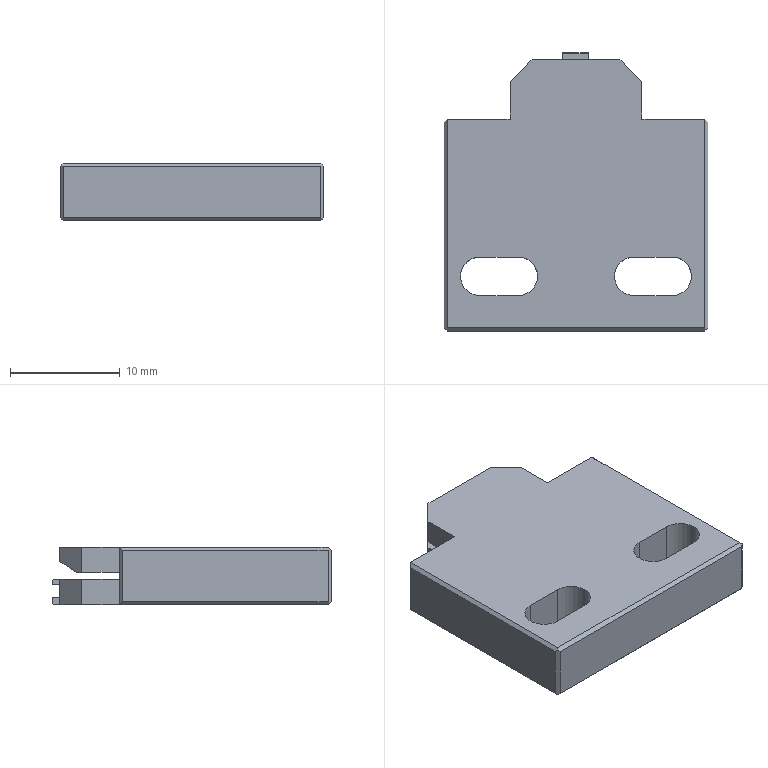Part | NX | 1 solid | 49 faces | box 24 x 25.342 x 5.25 mm | volume 2471 mm3 | plane 43 | cylinder 6 | commonest cylinder face diameters 3.5 x6
STEP:
#1=CARTESIAN_POINT('',(-1.2,-32.158,5.225));
#2=VERTEX_POINT('',#1);
#3=CARTESIAN_POINT('',(1.1,-32.158,5.225));
#4=VERTEX_POINT('',#3);
#5=CARTESIAN_POINT('',(-0.05,-32.158,5.225));
#6=DIRECTION('',(1.,0.,0.));
#7=VECTOR('',#6,1000.);
#8=LINE('',#5,#7);
#9=EDGE_CURVE('',#2,#4,#8,.T.);
#10=ORIENTED_EDGE('',*,*,#9,.T.);
#11=CARTESIAN_POINT('',(1.1,-32.158,4.822));
#12=VERTEX_POINT('',#11);
#13=CARTESIAN_POINT('',(1.1,-32.158,0.));
#14=DIRECTION('',(0.,0.,1.));
#15=VECTOR('',#14,1000.);
#16=LINE('',#13,#15);
#17=EDGE_CURVE('',#12,#4,#16,.T.);
#18=ORIENTED_EDGE('',*,*,#17,.F.);
#19=CARTESIAN_POINT('',(-1.2,-32.158,4.822));
#20=VERTEX_POINT('',#19);
#21=CARTESIAN_POINT('',(0.,-32.158,4.822));
#22=DIRECTION('',(-1.,0.,0.));
#23=VECTOR('',#22,1000.);
#24=LINE('',#21,#23);
#25=EDGE_CURVE('',#12,#20,#24,.T.);
#26=ORIENTED_EDGE('',*,*,#25,.T.);
#27=CARTESIAN_POINT('',(-1.2,-32.158,0.));
#28=DIRECTION('',(0.,0.,-1.));
#29=VECTOR('',#28,1000.);
#30=LINE('',#27,#29);
#31=EDGE_CURVE('',#2,#20,#30,.T.);
#32=ORIENTED_EDGE('',*,*,#31,.F.);
#33=EDGE_LOOP('',(#10,#18,#26,#32));
#34=FACE_BOUND('',#33,.T.);
#35=CARTESIAN_POINT('',(-4.2,-32.158,8.775));
#36=DIRECTION('',(0.,-1.,0.));
#37=DIRECTION('',(-1.,0.,0.));
#38=AXIS2_PLACEMENT_3D('',#35,#36,#37);
#39=PLANE('',#38);
#40=ADVANCED_FACE('',(#34),#39,.F.);
#41=ORIENTED_EDGE('',*,*,#9,.F.);
#42=CARTESIAN_POINT('',(-1.2,-32.258,5.325));
#43=VERTEX_POINT('',#42);
#44=CARTESIAN_POINT('',(-1.2,0.,-26.933));
#45=DIRECTION('',(0.,0.7071,-0.7071));
#46=VECTOR('',#45,1000.);
#47=LINE('',#44,#46);
#48=EDGE_CURVE('',#43,#2,#47,.T.);
#49=ORIENTED_EDGE('',*,*,#48,.F.);
#50=CARTESIAN_POINT('',(1.1,-32.258,5.325));
#51=VERTEX_POINT('',#50);
#52=CARTESIAN_POINT('',(-0.05,-32.258,5.325));
#53=DIRECTION('',(1.,0.,0.));
#54=VECTOR('',#53,1000.);
#55=LINE('',#52,#54);
#56=EDGE_CURVE('',#43,#51,#55,.T.);
#57=ORIENTED_EDGE('',*,*,#56,.T.);
#58=CARTESIAN_POINT('',(1.1,0.,-26.933));
#59=DIRECTION('',(0.,-0.7071,0.7071));
#60=VECTOR('',#59,1000.);
#61=LINE('',#58,#60);
#62=EDGE_CURVE('',#4,#51,#61,.T.);
#63=ORIENTED_EDGE('',*,*,#62,.F.);
#64=EDGE_LOOP('',(#41,#49,#57,#63));
#65=FACE_BOUND('',#64,.T.);
#66=CARTESIAN_POINT('',(-0.05,-32.208,5.275));
#67=DIRECTION('',(0.,0.7071,0.7071));
#68=DIRECTION('',(1.,0.,0.));
#69=AXIS2_PLACEMENT_3D('',#66,#67,#68);
#70=PLANE('',#69);
#71=ADVANCED_FACE('',(#65),#70,.T.);
#72=CARTESIAN_POINT('',(1.1,-32.158,3.1));
#73=VERTEX_POINT('',#72);
#74=CARTESIAN_POINT('',(-1.2,-32.158,3.1));
#75=VERTEX_POINT('',#74);
#76=CARTESIAN_POINT('',(-0.05,-32.158,3.1));
#77=DIRECTION('',(-1.,0.,0.));
#78=VECTOR('',#77,1000.);
#79=LINE('',#76,#78);
#80=EDGE_CURVE('',#73,#75,#79,.T.);
#81=ORIENTED_EDGE('',*,*,#80,.T.);
#82=CARTESIAN_POINT('',(-1.2,-32.158,3.7));
#83=VERTEX_POINT('',#82);
#84=CARTESIAN_POINT('',(-1.2,-32.158,0.));
#85=DIRECTION('',(0.,0.,-1.));
#86=VECTOR('',#85,1000.);
#87=LINE('',#84,#86);
#88=EDGE_CURVE('',#83,#75,#87,.T.);
#89=ORIENTED_EDGE('',*,*,#88,.F.);
#90=CARTESIAN_POINT('',(1.1,-32.158,3.7));
#91=VERTEX_POINT('',#90);
#92=CARTESIAN_POINT('',(0.,-32.158,3.7));
#93=DIRECTION('',(1.,0.,0.));
#94=VECTOR('',#93,1000.);
#95=LINE('',#92,#94);
#96=EDGE_CURVE('',#83,#91,#95,.T.);
#97=ORIENTED_EDGE('',*,*,#96,.T.);
#98=CARTESIAN_POINT('',(1.1,-32.158,0.));
#99=DIRECTION('',(0.,0.,1.));
#100=VECTOR('',#99,1000.);
#101=LINE('',#98,#100);
#102=EDGE_CURVE('',#73,#91,#101,.T.);
#103=ORIENTED_EDGE('',*,*,#102,.F.);
#104=EDGE_LOOP('',(#81,#89,#97,#103));
#105=FACE_BOUND('',#104,.T.);
#106=CARTESIAN_POINT('',(0.,-32.158,4.111));
#107=DIRECTION('',(0.,1.,0.));
#108=DIRECTION('',(1.,0.,0.));
#109=AXIS2_PLACEMENT_3D('',#106,#107,#108);
#110=PLANE('',#109);
#111=ADVANCED_FACE('',(#105),#110,.T.);
#112=ORIENTED_EDGE('',*,*,#80,.F.);
#113=CARTESIAN_POINT('',(1.1,-32.258,3.));
#114=VERTEX_POINT('',#113);
#115=CARTESIAN_POINT('',(1.1,0.,35.258));
#116=DIRECTION('',(0.,0.7071,0.7071));
#117=VECTOR('',#116,1000.);
#118=LINE('',#115,#117);
#119=EDGE_CURVE('',#114,#73,#118,.T.);
#120=ORIENTED_EDGE('',*,*,#119,.F.);
#121=CARTESIAN_POINT('',(-1.2,-32.258,3.));
#122=VERTEX_POINT('',#121);
#123=CARTESIAN_POINT('',(-0.05,-32.258,3.));
#124=DIRECTION('',(-1.,0.,0.));
#125=VECTOR('',#124,1000.);
#126=LINE('',#123,#125);
#127=EDGE_CURVE('',#114,#122,#126,.T.);
#128=ORIENTED_EDGE('',*,*,#127,.T.);
#129=CARTESIAN_POINT('',(-1.2,0.,35.258));
#130=DIRECTION('',(0.,-0.7071,-0.7071));
#131=VECTOR('',#130,1000.);
#132=LINE('',#129,#131);
#133=EDGE_CURVE('',#75,#122,#132,.T.);
#134=ORIENTED_EDGE('',*,*,#133,.F.);
#135=EDGE_LOOP('',(#112,#120,#128,#134));
#136=FACE_BOUND('',#135,.T.);
#137=CARTESIAN_POINT('',(-0.05,-32.208,3.05));
#138=DIRECTION('',(0.,0.7071,-0.7071));
#139=DIRECTION('',(-1.,0.,0.));
#140=AXIS2_PLACEMENT_3D('',#137,#138,#139);
#141=PLANE('',#140);
#142=ADVANCED_FACE('',(#136),#141,.T.);
#143=ORIENTED_EDGE('',*,*,#102,.T.);
#144=CARTESIAN_POINT('',(1.1,-32.815,3.7));
#145=VERTEX_POINT('',#144);
#146=CARTESIAN_POINT('',(1.1,0.,3.7));
#147=DIRECTION('',(0.,-1.,0.));
#148=VECTOR('',#147,1000.);
#149=LINE('',#146,#148);
#150=EDGE_CURVE('',#91,#145,#149,.T.);
#151=ORIENTED_EDGE('',*,*,#150,.T.);
#152=CARTESIAN_POINT('',(1.1,-32.815,3.));
#153=VERTEX_POINT('',#152);
#154=CARTESIAN_POINT('',(1.1,-32.815,0.));
#155=DIRECTION('',(0.,0.,1.));
#156=VECTOR('',#155,1000.);
#157=LINE('',#154,#156);
#158=EDGE_CURVE('',#153,#145,#157,.T.);
#159=ORIENTED_EDGE('',*,*,#158,.F.);
#160=CARTESIAN_POINT('',(1.1,0.,3.));
#161=DIRECTION('',(0.,1.,0.));
#162=VECTOR('',#161,1000.);
#163=LINE('',#160,#162);
#164=EDGE_CURVE('',#153,#114,#163,.T.);
#165=ORIENTED_EDGE('',*,*,#164,.T.);
#166=ORIENTED_EDGE('',*,*,#119,.T.);
#167=EDGE_LOOP('',(#143,#151,#159,#165,#166));
#168=FACE_BOUND('',#167,.T.);
#169=CARTESIAN_POINT('',(1.1,-33.565,2.475));
#170=DIRECTION('',(-1.,0.,0.));
#171=DIRECTION('',(0.,0.,1.));
#172=AXIS2_PLACEMENT_3D('',#169,#170,#171);
#173=PLANE('',#172);
#174=ADVANCED_FACE('',(#168),#173,.F.);
#175=ORIENTED_EDGE('',*,*,#150,.F.);
#176=ORIENTED_EDGE('',*,*,#96,.F.);
#177=CARTESIAN_POINT('',(-1.2,-32.815,3.7));
#178=VERTEX_POINT('',#177);
#179=CARTESIAN_POINT('',(-1.2,0.,3.7));
#180=DIRECTION('',(0.,1.,0.));
#181=VECTOR('',#180,1000.);
#182=LINE('',#179,#181);
#183=EDGE_CURVE('',#178,#83,#182,.T.);
#184=ORIENTED_EDGE('',*,*,#183,.F.);
#185=CARTESIAN_POINT('',(0.,-32.815,3.7));
#186=DIRECTION('',(-1.,0.,0.));
#187=VECTOR('',#186,1000.);
#188=LINE('',#185,#187);
#189=EDGE_CURVE('',#145,#178,#188,.T.);
#190=ORIENTED_EDGE('',*,*,#189,.F.);
#191=EDGE_LOOP('',(#175,#176,#184,#190));
#192=FACE_BOUND('',#191,.T.);
#193=CARTESIAN_POINT('',(6.,-34.,3.7));
#194=DIRECTION('',(0.,0.,1.));
#195=DIRECTION('',(0.,-1.,0.));
#196=AXIS2_PLACEMENT_3D('',#193,#194,#195);
#197=PLANE('',#196);
#198=ADVANCED_FACE('',(#192),#197,.T.);
#199=CARTESIAN_POINT('',(-4.,-32.815,5.325));
#200=VERTEX_POINT('',#199);
#201=CARTESIAN_POINT('',(-4.,-32.815,3.));
#202=VERTEX_POINT('',#201);
#203=CARTESIAN_POINT('',(-4.,-32.815,4.175));
#204=DIRECTION('',(0.,0.,-1.));
#205=VECTOR('',#204,1000.);
#206=LINE('',#203,#205);
#207=EDGE_CURVE('',#200,#202,#206,.T.);
#208=ORIENTED_EDGE('',*,*,#207,.F.);
#209=CARTESIAN_POINT('',(-1.2,-32.815,5.325));
#210=VERTEX_POINT('',#209);
#211=CARTESIAN_POINT('',(0.,-32.815,5.325));
#212=DIRECTION('',(1.,0.,0.));
#213=VECTOR('',#212,1000.);
#214=LINE('',#211,#213);
#215=EDGE_CURVE('',#200,#210,#214,.T.);
#216=ORIENTED_EDGE('',*,*,#215,.T.);
#217=CARTESIAN_POINT('',(-1.2,-32.815,4.822));
#218=VERTEX_POINT('',#217);
#219=CARTESIAN_POINT('',(-1.2,-32.815,0.));
#220=DIRECTION('',(0.,0.,-1.));
#221=VECTOR('',#220,1000.);
#222=LINE('',#219,#221);
#223=EDGE_CURVE('',#210,#218,#222,.T.);
#224=ORIENTED_EDGE('',*,*,#223,.T.);
#225=CARTESIAN_POINT('',(1.1,-32.815,4.822));
#226=VERTEX_POINT('',#225);
#227=CARTESIAN_POINT('',(0.,-32.815,4.822));
#228=DIRECTION('',(1.,0.,0.));
#229=VECTOR('',#228,1000.);
#230=LINE('',#227,#229);
#231=EDGE_CURVE('',#218,#226,#230,.T.);
#232=ORIENTED_EDGE('',*,*,#231,.T.);
#233=CARTESIAN_POINT('',(1.1,-32.815,5.325));
#234=VERTEX_POINT('',#233);
#235=CARTESIAN_POINT('',(1.1,-32.815,0.));
#236=DIRECTION('',(0.,0.,-1.));
#237=VECTOR('',#236,1000.);
#238=LINE('',#235,#237);
#239=EDGE_CURVE('',#234,#226,#238,.T.);
#240=ORIENTED_EDGE('',*,*,#239,.F.);
#241=CARTESIAN_POINT('',(4.,-32.815,5.325));
#242=VERTEX_POINT('',#241);
#243=CARTESIAN_POINT('',(0.,-32.815,5.325));
#244=DIRECTION('',(1.,0.,0.));
#245=VECTOR('',#244,1000.);
#246=LINE('',#243,#245);
#247=EDGE_CURVE('',#234,#242,#246,.T.);
#248=ORIENTED_EDGE('',*,*,#247,.T.);
#249=CARTESIAN_POINT('',(4.,-32.815,3.));
#250=VERTEX_POINT('',#249);
#251=CARTESIAN_POINT('',(4.,-32.815,4.175));
#252=DIRECTION('',(0.,0.,1.));
#253=VECTOR('',#252,1000.);
#254=LINE('',#251,#253);
#255=EDGE_CURVE('',#250,#242,#254,.T.);
#256=ORIENTED_EDGE('',*,*,#255,.F.);
#257=CARTESIAN_POINT('',(0.,-32.815,3.));
#258=DIRECTION('',(-1.,0.,0.));
#259=VECTOR('',#258,1000.);
#260=LINE('',#257,#259);
#261=EDGE_CURVE('',#250,#153,#260,.T.);
#262=ORIENTED_EDGE('',*,*,#261,.T.);
#263=ORIENTED_EDGE('',*,*,#158,.T.);
#264=ORIENTED_EDGE('',*,*,#189,.T.);
#265=CARTESIAN_POINT('',(-1.2,-32.815,3.));
#266=VERTEX_POINT('',#265);
#267=CARTESIAN_POINT('',(-1.2,-32.815,0.));
#268=DIRECTION('',(0.,0.,-1.));
#269=VECTOR('',#268,1000.);
#270=LINE('',#267,#269);
#271=EDGE_CURVE('',#178,#266,#270,.T.);
#272=ORIENTED_EDGE('',*,*,#271,.T.);
#273=CARTESIAN_POINT('',(0.,-32.815,3.));
#274=DIRECTION('',(-1.,0.,0.));
#275=VECTOR('',#274,1000.);
#276=LINE('',#273,#275);
#277=EDGE_CURVE('',#266,#202,#276,.T.);
#278=ORIENTED_EDGE('',*,*,#277,.T.);
#279=EDGE_LOOP('',(#208,#216,#224,#232,#240,#248,#256,#262,#263,#264,#272,#278));
#280=FACE_BOUND('',#279,.T.);
#281=CARTESIAN_POINT('',(6.,-32.815,2.475));
#282=DIRECTION('',(0.,-1.,0.));
#283=DIRECTION('',(0.,0.,-1.));
#284=AXIS2_PLACEMENT_3D('',#281,#282,#283);
#285=PLANE('',#284);
#286=ADVANCED_FACE('',(#280),#285,.F.);
#287=CARTESIAN_POINT('',(11.7,-38.2,3.));
#288=VERTEX_POINT('',#287);
#289=CARTESIAN_POINT('',(11.7,-57.2,3.));
#290=VERTEX_POINT('',#289);
#291=CARTESIAN_POINT('',(11.7,-47.85,3.));
#292=DIRECTION('',(0.,-1.,0.));
#293=VECTOR('',#292,1000.);
#294=LINE('',#291,#293);
#295=EDGE_CURVE('',#288,#290,#294,.T.);
#296=ORIENTED_EDGE('',*,*,#295,.T.);
#297=CARTESIAN_POINT('',(-11.7,-57.2,3.));
#298=VERTEX_POINT('',#297);
#299=CARTESIAN_POINT('',(0.,-57.2,3.));
#300=DIRECTION('',(1.,0.,0.));
#301=VECTOR('',#300,1000.);
#302=LINE('',#299,#301);
#303=EDGE_CURVE('',#298,#290,#302,.T.);
#304=ORIENTED_EDGE('',*,*,#303,.F.);
#305=CARTESIAN_POINT('',(-11.7,-38.2,3.));
#306=VERTEX_POINT('',#305);
#307=CARTESIAN_POINT('',(-11.7,-47.85,3.));
#308=DIRECTION('',(0.,-1.,0.));
#309=VECTOR('',#308,1000.);
#310=LINE('',#307,#309);
#311=EDGE_CURVE('',#306,#298,#310,.T.);
#312=ORIENTED_EDGE('',*,*,#311,.F.);
#313=CARTESIAN_POINT('',(-6.,-38.2,3.));
#314=VERTEX_POINT('',#313);
#315=CARTESIAN_POINT('',(0.,-38.2,3.));
#316=DIRECTION('',(-1.,0.,0.));
#317=VECTOR('',#316,1000.);
#318=LINE('',#315,#317);
#319=EDGE_CURVE('',#314,#306,#318,.T.);
#320=ORIENTED_EDGE('',*,*,#319,.F.);
#321=CARTESIAN_POINT('',(-6.,-34.815,3.));
#322=VERTEX_POINT('',#321);
#323=CARTESIAN_POINT('',(-6.,-33.565,3.));
#324=DIRECTION('',(0.,1.,0.));
#325=VECTOR('',#324,1000.);
#326=LINE('',#323,#325);
#327=EDGE_CURVE('',#314,#322,#326,.T.);
#328=ORIENTED_EDGE('',*,*,#327,.T.);
#329=CARTESIAN_POINT('',(28.815,0.,3.));
#330=DIRECTION('',(0.7071,0.7071,0.));
#331=VECTOR('',#330,1000.);
#332=LINE('',#329,#331);
#333=EDGE_CURVE('',#322,#202,#332,.T.);
#334=ORIENTED_EDGE('',*,*,#333,.T.);
#335=ORIENTED_EDGE('',*,*,#277,.F.);
#336=CARTESIAN_POINT('',(-1.2,0.,3.));
#337=DIRECTION('',(0.,-1.,0.));
#338=VECTOR('',#337,1000.);
#339=LINE('',#336,#338);
#340=EDGE_CURVE('',#122,#266,#339,.T.);
#341=ORIENTED_EDGE('',*,*,#340,.F.);
#342=ORIENTED_EDGE('',*,*,#127,.F.);
#343=ORIENTED_EDGE('',*,*,#164,.F.);
#344=ORIENTED_EDGE('',*,*,#261,.F.);
#345=CARTESIAN_POINT('',(6.,-34.815,3.));
#346=VERTEX_POINT('',#345);
#347=CARTESIAN_POINT('',(-28.815,0.,3.));
#348=DIRECTION('',(-0.7071,0.7071,0.));
#349=VECTOR('',#348,1000.);
#350=LINE('',#347,#349);
#351=EDGE_CURVE('',#346,#250,#350,.T.);
#352=ORIENTED_EDGE('',*,*,#351,.F.);
#353=CARTESIAN_POINT('',(6.,-38.2,3.));
#354=VERTEX_POINT('',#353);
#355=CARTESIAN_POINT('',(6.,0.,3.));
#356=DIRECTION('',(0.,1.,0.));
#357=VECTOR('',#356,1000.);
#358=LINE('',#355,#357);
#359=EDGE_CURVE('',#354,#346,#358,.T.);
#360=ORIENTED_EDGE('',*,*,#359,.F.);
#361=CARTESIAN_POINT('',(0.,-38.2,3.));
#362=DIRECTION('',(-1.,0.,0.));
#363=VECTOR('',#362,1000.);
#364=LINE('',#361,#363);
#365=EDGE_CURVE('',#288,#354,#364,.T.);
#366=ORIENTED_EDGE('',*,*,#365,.F.);
#367=EDGE_LOOP('',(#296,#304,#312,#320,#328,#334,#335,#341,#342,#343,#344,#352,#360,#366));
#368=FACE_BOUND('',#367,.T.);
#369=CARTESIAN_POINT('',(8.75,-54.25,3.));
#370=VERTEX_POINT('',#369);
#371=CARTESIAN_POINT('',(5.25,-54.25,3.));
#372=VERTEX_POINT('',#371);
#373=CARTESIAN_POINT('',(0.,-54.25,3.));
#374=DIRECTION('',(-1.,0.,0.));
#375=VECTOR('',#374,1000.);
#376=LINE('',#373,#375);
#377=EDGE_CURVE('',#370,#372,#376,.T.);
#378=ORIENTED_EDGE('',*,*,#377,.F.);
#379=CARTESIAN_POINT('',(10.5,-52.5,3.));
#380=VERTEX_POINT('',#379);
#381=CARTESIAN_POINT('',(8.75,-52.5,3.));
#382=DIRECTION('',(0.,0.,1.));
#383=DIRECTION('',(1.,0.,0.));
#384=AXIS2_PLACEMENT_3D('',#381,#382,#383);
#385=CIRCLE('',#384,1.75);
#386=EDGE_CURVE('',#370,#380,#385,.T.);
#387=ORIENTED_EDGE('',*,*,#386,.T.);
#388=CARTESIAN_POINT('',(8.75,-50.75,3.));
#389=VERTEX_POINT('',#388);
#390=CARTESIAN_POINT('',(8.75,-52.5,3.));
#391=DIRECTION('',(0.,0.,1.));
#392=DIRECTION('',(1.,0.,0.));
#393=AXIS2_PLACEMENT_3D('',#390,#391,#392);
#394=CIRCLE('',#393,1.75);
#395=EDGE_CURVE('',#380,#389,#394,.T.);
#396=ORIENTED_EDGE('',*,*,#395,.T.);
#397=CARTESIAN_POINT('',(5.25,-50.75,3.));
#398=VERTEX_POINT('',#397);
#399=CARTESIAN_POINT('',(0.,-50.75,3.));
#400=DIRECTION('',(1.,0.,0.));
#401=VECTOR('',#400,1000.);
#402=LINE('',#399,#401);
#403=EDGE_CURVE('',#398,#389,#402,.T.);
#404=ORIENTED_EDGE('',*,*,#403,.F.);
#405=CARTESIAN_POINT('',(5.25,-52.5,3.));
#406=DIRECTION('',(0.,0.,1.));
#407=DIRECTION('',(1.,0.,0.));
#408=AXIS2_PLACEMENT_3D('',#405,#406,#407);
#409=CIRCLE('',#408,1.75);
#410=EDGE_CURVE('',#398,#372,#409,.T.);
#411=ORIENTED_EDGE('',*,*,#410,.T.);
#412=EDGE_LOOP('',(#378,#387,#396,#404,#411));
#413=FACE_BOUND('',#412,.T.);
#414=CARTESIAN_POINT('',(-5.25,-54.25,3.));
#415=VERTEX_POINT('',#414);
#416=CARTESIAN_POINT('',(-8.75,-54.25,3.));
#417=VERTEX_POINT('',#416);
#418=CARTESIAN_POINT('',(0.,-54.25,3.));
#419=DIRECTION('',(-1.,0.,0.));
#420=VECTOR('',#419,1000.);
#421=LINE('',#418,#420);
#422=EDGE_CURVE('',#415,#417,#421,.T.);
#423=ORIENTED_EDGE('',*,*,#422,.F.);
#424=CARTESIAN_POINT('',(-3.5,-52.5,3.));
#425=VERTEX_POINT('',#424);
#426=CARTESIAN_POINT('',(-5.25,-52.5,3.));
#427=DIRECTION('',(0.,0.,1.));
#428=DIRECTION('',(1.,0.,0.));
#429=AXIS2_PLACEMENT_3D('',#426,#427,#428);
#430=CIRCLE('',#429,1.75);
#431=EDGE_CURVE('',#415,#425,#430,.T.);
#432=ORIENTED_EDGE('',*,*,#431,.T.);
#433=CARTESIAN_POINT('',(-5.25,-50.75,3.));
#434=VERTEX_POINT('',#433);
#435=CARTESIAN_POINT('',(-5.25,-52.5,3.));
#436=DIRECTION('',(0.,0.,1.));
#437=DIRECTION('',(1.,0.,0.));
#438=AXIS2_PLACEMENT_3D('',#435,#436,#437);
#439=CIRCLE('',#438,1.75);
#440=EDGE_CURVE('',#425,#434,#439,.T.);
#441=ORIENTED_EDGE('',*,*,#440,.T.);
#442=CARTESIAN_POINT('',(-8.75,-50.75,3.));
#443=VERTEX_POINT('',#442);
#444=CARTESIAN_POINT('',(0.,-50.75,3.));
#445=DIRECTION('',(1.,0.,0.));
#446=VECTOR('',#445,1000.);
#447=LINE('',#444,#446);
#448=EDGE_CURVE('',#443,#434,#447,.T.);
#449=ORIENTED_EDGE('',*,*,#448,.F.);
#450=CARTESIAN_POINT('',(-8.75,-52.5,3.));
#451=DIRECTION('',(0.,0.,1.));
#452=DIRECTION('',(1.,0.,0.));
#453=AXIS2_PLACEMENT_3D('',#450,#451,#452);
#454=CIRCLE('',#453,1.75);
#455=EDGE_CURVE('',#443,#417,#454,.T.);
#456=ORIENTED_EDGE('',*,*,#455,.T.);
#457=EDGE_LOOP('',(#423,#432,#441,#449,#456));
#458=FACE_BOUND('',#457,.T.);
#459=CARTESIAN_POINT('',(1.4,-33.565,3.));
#460=DIRECTION('',(0.,0.,-1.));
#461=DIRECTION('',(-1.,0.,0.));
#462=AXIS2_PLACEMENT_3D('',#459,#460,#461);
#463=PLANE('',#462);
#464=ADVANCED_FACE('',(#368,#413,#458),#463,.T.);
#465=CARTESIAN_POINT('',(10.5,-52.5,8.25));
#466=VERTEX_POINT('',#465);
#467=CARTESIAN_POINT('',(10.5,-52.5,2.475));
#468=DIRECTION('',(0.,0.,1.));
#469=VECTOR('',#468,1000.);
#470=LINE('',#467,#469);
#471=EDGE_CURVE('',#380,#466,#470,.T.);
#472=ORIENTED_EDGE('',*,*,#471,.F.);
#473=ORIENTED_EDGE('',*,*,#386,.F.);
#474=CARTESIAN_POINT('',(8.75,-54.25,8.25));
#475=VERTEX_POINT('',#474);
#476=CARTESIAN_POINT('',(8.75,-54.25,2.475));
#477=DIRECTION('',(0.,0.,1.));
#478=VECTOR('',#477,1000.);
#479=LINE('',#476,#478);
#480=EDGE_CURVE('',#370,#475,#479,.T.);
#481=ORIENTED_EDGE('',*,*,#480,.T.);
#482=CARTESIAN_POINT('',(8.75,-52.5,8.25));
#483=DIRECTION('',(0.,0.,1.));
#484=DIRECTION('',(1.,0.,0.));
#485=AXIS2_PLACEMENT_3D('',#482,#483,#484);
#486=CIRCLE('',#485,1.75);
#487=EDGE_CURVE('',#475,#466,#486,.T.);
#488=ORIENTED_EDGE('',*,*,#487,.T.);
#489=EDGE_LOOP('',(#472,#473,#481,#488));
#490=FACE_BOUND('',#489,.T.);
#491=CARTESIAN_POINT('',(8.75,-52.5,2.475));
#492=DIRECTION('',(0.,0.,1.));
#493=DIRECTION('',(1.,0.,0.));
#494=AXIS2_PLACEMENT_3D('',#491,#492,#493);
#495=CYLINDRICAL_SURFACE('',#494,1.75);
#496=ADVANCED_FACE('',(#490),#495,.F.);
#497=CARTESIAN_POINT('',(8.75,-50.75,8.25));
#498=VERTEX_POINT('',#497);
#499=CARTESIAN_POINT('',(5.25,-50.75,8.25));
#500=VERTEX_POINT('',#499);
#501=CARTESIAN_POINT('',(0.,-50.75,8.25));
#502=DIRECTION('',(-1.,0.,0.));
#503=VECTOR('',#502,1000.);
#504=LINE('',#501,#503);
#505=EDGE_CURVE('',#498,#500,#504,.T.);
#506=ORIENTED_EDGE('',*,*,#505,.T.);
#507=CARTESIAN_POINT('',(5.25,-50.75,2.475));
#508=DIRECTION('',(0.,0.,1.));
#509=VECTOR('',#508,1000.);
#510=LINE('',#507,#509);
#511=EDGE_CURVE('',#398,#500,#510,.T.);
#512=ORIENTED_EDGE('',*,*,#511,.F.);
#513=ORIENTED_EDGE('',*,*,#403,.T.);
#514=CARTESIAN_POINT('',(8.75,-50.75,2.475));
#515=DIRECTION('',(0.,0.,1.));
#516=VECTOR('',#515,1000.);
#517=LINE('',#514,#516);
#518=EDGE_CURVE('',#389,#498,#517,.T.);
#519=ORIENTED_EDGE('',*,*,#518,.T.);
#520=EDGE_LOOP('',(#506,#512,#513,#519));
#521=FACE_BOUND('',#520,.T.);
#522=CARTESIAN_POINT('',(5.25,-50.75,2.475));
#523=DIRECTION('',(0.,1.,0.));
#524=DIRECTION('',(1.,0.,0.));
#525=AXIS2_PLACEMENT_3D('',#522,#523,#524);
#526=PLANE('',#525);
#527=ADVANCED_FACE('',(#521),#526,.F.);
#528=ORIENTED_EDGE('',*,*,#377,.T.);
#529=CARTESIAN_POINT('',(5.25,-54.25,8.25));
#530=VERTEX_POINT('',#529);
#531=CARTESIAN_POINT('',(5.25,-54.25,2.475));
#532=DIRECTION('',(0.,0.,1.));
#533=VECTOR('',#532,1000.);
#534=LINE('',#531,#533);
#535=EDGE_CURVE('',#372,#530,#534,.T.);
#536=ORIENTED_EDGE('',*,*,#535,.T.);
#537=CARTESIAN_POINT('',(0.,-54.25,8.25));
#538=DIRECTION('',(1.,0.,0.));
#539=VECTOR('',#538,1000.);
#540=LINE('',#537,#539);
#541=EDGE_CURVE('',#530,#475,#540,.T.);
#542=ORIENTED_EDGE('',*,*,#541,.T.);
#543=ORIENTED_EDGE('',*,*,#480,.F.);
#544=EDGE_LOOP('',(#528,#536,#542,#543));
#545=FACE_BOUND('',#544,.T.);
#546=CARTESIAN_POINT('',(8.75,-54.25,2.475));
#547=DIRECTION('',(0.,-1.,0.));
#548=DIRECTION('',(0.,0.,-1.));
#549=AXIS2_PLACEMENT_3D('',#546,#547,#548);
#550=PLANE('',#549);
#551=ADVANCED_FACE('',(#545),#550,.F.);
#552=ORIENTED_EDGE('',*,*,#410,.F.);
#553=ORIENTED_EDGE('',*,*,#511,.T.);
#554=CARTESIAN_POINT('',(5.25,-52.5,8.25));
#555=DIRECTION('',(0.,0.,1.));
#556=DIRECTION('',(1.,0.,0.));
#557=AXIS2_PLACEMENT_3D('',#554,#555,#556);
#558=CIRCLE('',#557,1.75);
#559=EDGE_CURVE('',#500,#530,#558,.T.);
#560=ORIENTED_EDGE('',*,*,#559,.T.);
#561=ORIENTED_EDGE('',*,*,#535,.F.);
#562=EDGE_LOOP('',(#552,#553,#560,#561));
#563=FACE_BOUND('',#562,.T.);
#564=CARTESIAN_POINT('',(5.25,-52.5,2.475));
#565=DIRECTION('',(0.,0.,1.));
#566=DIRECTION('',(1.,0.,0.));
#567=AXIS2_PLACEMENT_3D('',#564,#565,#566);
#568=CYLINDRICAL_SURFACE('',#567,1.75);
#569=ADVANCED_FACE('',(#563),#568,.F.);
#570=ORIENTED_EDGE('',*,*,#207,.T.);
#571=ORIENTED_EDGE('',*,*,#333,.F.);
#572=CARTESIAN_POINT('',(-6.,-34.815,5.325));
#573=VERTEX_POINT('',#572);
#574=CARTESIAN_POINT('',(-6.,-34.815,4.175));
#575=DIRECTION('',(0.,0.,-1.));
#576=VECTOR('',#575,1000.);
#577=LINE('',#574,#576);
#578=EDGE_CURVE('',#573,#322,#577,.T.);
#579=ORIENTED_EDGE('',*,*,#578,.F.);
#580=CARTESIAN_POINT('',(28.815,0.,5.325));
#581=DIRECTION('',(0.7071,0.7071,0.));
#582=VECTOR('',#581,1000.);
#583=LINE('',#580,#582);
#584=EDGE_CURVE('',#573,#200,#583,.T.);
#585=ORIENTED_EDGE('',*,*,#584,.T.);
#586=EDGE_LOOP('',(#570,#571,#579,#585));
#587=FACE_BOUND('',#586,.T.);
#588=CARTESIAN_POINT('',(-5.,-33.815,4.175));
#589=DIRECTION('',(0.7071,-0.7071,0.));
#590=DIRECTION('',(0.,0.,-1.));
#591=AXIS2_PLACEMENT_3D('',#588,#589,#590);
#592=PLANE('',#591);
#593=ADVANCED_FACE('',(#587),#592,.F.);
#594=CARTESIAN_POINT('',(1.1,0.,5.325));
#595=DIRECTION('',(0.,-1.,0.));
#596=VECTOR('',#595,1000.);
#597=LINE('',#594,#596);
#598=EDGE_CURVE('',#51,#234,#597,.T.);
#599=ORIENTED_EDGE('',*,*,#598,.T.);
#600=ORIENTED_EDGE('',*,*,#239,.T.);
#601=CARTESIAN_POINT('',(1.1,-32.258,4.822));
#602=DIRECTION('',(0.,1.,0.));
#603=VECTOR('',#602,1000.);
#604=LINE('',#601,#603);
#605=EDGE_CURVE('',#226,#12,#604,.T.);
#606=ORIENTED_EDGE('',*,*,#605,.T.);
#607=ORIENTED_EDGE('',*,*,#17,.T.);
#608=ORIENTED_EDGE('',*,*,#62,.T.);
#609=EDGE_LOOP('',(#599,#600,#606,#607,#608));
#610=FACE_BOUND('',#609,.T.);
#611=CARTESIAN_POINT('',(1.1,-30.615,8.775));
#612=DIRECTION('',(-1.,0.,0.));
#613=DIRECTION('',(0.,0.,1.));
#614=AXIS2_PLACEMENT_3D('',#611,#612,#613);
#615=PLANE('',#614);
#616=ADVANCED_FACE('',(#610),#615,.F.);
#617=ORIENTED_EDGE('',*,*,#295,.F.);
#618=CARTESIAN_POINT('',(12.,-38.5,3.3));
#619=VERTEX_POINT('',#618);
#620=CARTESIAN_POINT('',(0.,-26.5,-8.7));
#621=DIRECTION('',(-0.5774,0.5774,-0.5774));
#622=VECTOR('',#621,1000.);
#623=LINE('',#620,#622);
#624=EDGE_CURVE('',#619,#288,#623,.T.);
#625=ORIENTED_EDGE('',*,*,#624,.F.);
#626=CARTESIAN_POINT('',(12.,-57.2,3.3));
#627=VERTEX_POINT('',#626);
#628=CARTESIAN_POINT('',(12.,-47.85,3.3));
#629=DIRECTION('',(0.,-1.,0.));
#630=VECTOR('',#629,1000.);
#631=LINE('',#628,#630);
#632=EDGE_CURVE('',#619,#627,#631,.T.);
#633=ORIENTED_EDGE('',*,*,#632,.T.);
#634=CARTESIAN_POINT('',(11.85,-57.35,3.15));
#635=VERTEX_POINT('',#634);
#636=CARTESIAN_POINT('',(0.,-69.2,-8.7));
#637=DIRECTION('',(-0.5774,-0.5774,-0.5774));
#638=VECTOR('',#637,1000.);
#639=LINE('',#636,#638);
#640=EDGE_CURVE('',#627,#635,#639,.T.);
#641=ORIENTED_EDGE('',*,*,#640,.T.);
#642=CARTESIAN_POINT('',(0.,-45.5,-8.7));
#643=DIRECTION('',(0.5774,-0.5774,0.5774));
#644=VECTOR('',#643,1000.);
#645=LINE('',#642,#644);
#646=EDGE_CURVE('',#290,#635,#645,.T.);
#647=ORIENTED_EDGE('',*,*,#646,.F.);
#648=EDGE_LOOP('',(#617,#625,#633,#641,#647));
#649=FACE_BOUND('',#648,.T.);
#650=CARTESIAN_POINT('',(11.85,-47.85,3.15));
#651=DIRECTION('',(0.7071,0.,-0.7071));
#652=DIRECTION('',(0.,-1.,0.));
#653=AXIS2_PLACEMENT_3D('',#650,#651,#652);
#654=PLANE('',#653);
#655=ADVANCED_FACE('',(#649),#654,.T.);
#656=CARTESIAN_POINT('',(-1.2,0.,4.822));
#657=DIRECTION('',(0.,-1.,0.));
#658=VECTOR('',#657,1000.);
#659=LINE('',#656,#658);
#660=EDGE_CURVE('',#20,#218,#659,.T.);
#661=ORIENTED_EDGE('',*,*,#660,.T.);
#662=ORIENTED_EDGE('',*,*,#223,.F.);
#663=CARTESIAN_POINT('',(-1.2,0.,5.325));
#664=DIRECTION('',(0.,1.,0.));
#665=VECTOR('',#664,1000.);
#666=LINE('',#663,#665);
#667=EDGE_CURVE('',#210,#43,#666,.T.);
#668=ORIENTED_EDGE('',*,*,#667,.T.);
#669=ORIENTED_EDGE('',*,*,#48,.T.);
#670=ORIENTED_EDGE('',*,*,#31,.T.);
#671=EDGE_LOOP('',(#661,#662,#668,#669,#670));
#672=FACE_BOUND('',#671,.T.);
#673=CARTESIAN_POINT('',(-1.2,-32.815,8.775));
#674=DIRECTION('',(1.,0.,0.));
#675=DIRECTION('',(0.,-1.,0.));
#676=AXIS2_PLACEMENT_3D('',#673,#674,#675);
#677=PLANE('',#676);
#678=ADVANCED_FACE('',(#672),#677,.F.);
#679=ORIENTED_EDGE('',*,*,#605,.F.);
#680=ORIENTED_EDGE('',*,*,#231,.F.);
#681=ORIENTED_EDGE('',*,*,#660,.F.);
#682=ORIENTED_EDGE('',*,*,#25,.F.);
#683=EDGE_LOOP('',(#679,#680,#681,#682));
#684=FACE_BOUND('',#683,.T.);
#685=CARTESIAN_POINT('',(-1.577,-32.815,4.822));
#686=DIRECTION('',(0.,0.,-1.));
#687=DIRECTION('',(-1.,0.,0.));
#688=AXIS2_PLACEMENT_3D('',#685,#686,#687);
#689=PLANE('',#688);
#690=ADVANCED_FACE('',(#684),#689,.T.);
#691=ORIENTED_EDGE('',*,*,#340,.T.);
#692=ORIENTED_EDGE('',*,*,#271,.F.);
#693=ORIENTED_EDGE('',*,*,#183,.T.);
#694=ORIENTED_EDGE('',*,*,#88,.T.);
#695=ORIENTED_EDGE('',*,*,#133,.T.);
#696=EDGE_LOOP('',(#691,#692,#693,#694,#695));
#697=FACE_BOUND('',#696,.T.);
#698=CARTESIAN_POINT('',(-1.2,-32.258,2.475));
#699=DIRECTION('',(1.,0.,0.));
#700=DIRECTION('',(0.,1.,0.));
#701=AXIS2_PLACEMENT_3D('',#698,#699,#700);
#702=PLANE('',#701);
#703=ADVANCED_FACE('',(#697),#702,.F.);
#704=CARTESIAN_POINT('',(5.5,-34.315,5.948));
#705=VERTEX_POINT('',#704);
#706=CARTESIAN_POINT('',(-5.5,-34.315,5.948));
#707=VERTEX_POINT('',#706);
#708=CARTESIAN_POINT('',(0.,-34.315,5.948));
#709=DIRECTION('',(-1.,0.,0.));
#710=VECTOR('',#709,1000.);
#711=LINE('',#708,#710);
#712=EDGE_CURVE('',#705,#707,#711,.T.);
#713=ORIENTED_EDGE('',*,*,#712,.F.);
#714=CARTESIAN_POINT('',(6.,-34.815,5.948));
#715=VERTEX_POINT('',#714);
#716=CARTESIAN_POINT('',(-28.815,0.,5.948));
#717=DIRECTION('',(-0.7071,0.7071,0.));
#718=VECTOR('',#717,1000.);
#719=LINE('',#716,#718);
#720=EDGE_CURVE('',#715,#705,#719,.T.);
#721=ORIENTED_EDGE('',*,*,#720,.F.);
#722=CARTESIAN_POINT('',(6.,-38.2,5.948));
#723=VERTEX_POINT('',#722);
#724=CARTESIAN_POINT('',(6.,0.,5.948));
#725=DIRECTION('',(0.,-1.,0.));
#726=VECTOR('',#725,1000.);
#727=LINE('',#724,#726);
#728=EDGE_CURVE('',#715,#723,#727,.T.);
#729=ORIENTED_EDGE('',*,*,#728,.T.);
#730=CARTESIAN_POINT('',(-6.,-38.2,5.948));
#731=VERTEX_POINT('',#730);
#732=CARTESIAN_POINT('',(0.,-38.2,5.948));
#733=DIRECTION('',(-1.,0.,0.));
#734=VECTOR('',#733,1000.);
#735=LINE('',#732,#734);
#736=EDGE_CURVE('',#723,#731,#735,.T.);
#737=ORIENTED_EDGE('',*,*,#736,.T.);
#738=CARTESIAN_POINT('',(-6.,-34.815,5.948));
#739=VERTEX_POINT('',#738);
#740=CARTESIAN_POINT('',(-6.,0.,5.948));
#741=DIRECTION('',(0.,-1.,0.));
#742=VECTOR('',#741,1000.);
#743=LINE('',#740,#742);
#744=EDGE_CURVE('',#739,#731,#743,.T.);
#745=ORIENTED_EDGE('',*,*,#744,.F.);
#746=CARTESIAN_POINT('',(28.815,0.,5.948));
#747=DIRECTION('',(0.7071,0.7071,0.));
#748=VECTOR('',#747,1000.);
#749=LINE('',#746,#748);
#750=EDGE_CURVE('',#739,#707,#749,.T.);
#751=ORIENTED_EDGE('',*,*,#750,.T.);
#752=EDGE_LOOP('',(#713,#721,#729,#737,#745,#751));
#753=FACE_BOUND('',#752,.T.);
#754=CARTESIAN_POINT('',(-0.02232,-30.694,5.948));
#755=DIRECTION('',(0.,0.,1.));
#756=DIRECTION('',(1.,0.,0.));
#757=AXIS2_PLACEMENT_3D('',#754,#755,#756);
#758=PLANE('',#757);
#759=ADVANCED_FACE('',(#753),#758,.F.);
#760=CARTESIAN_POINT('',(6.,-38.2,8.25));
#761=VERTEX_POINT('',#760);
#762=CARTESIAN_POINT('',(6.,-38.2,0.));
#763=DIRECTION('',(0.,0.,1.));
#764=VECTOR('',#763,1000.);
#765=LINE('',#762,#764);
#766=EDGE_CURVE('',#723,#761,#765,.T.);
#767=ORIENTED_EDGE('',*,*,#766,.T.);
#768=CARTESIAN_POINT('',(11.7,-38.2,8.25));
#769=VERTEX_POINT('',#768);
#770=CARTESIAN_POINT('',(0.,-38.2,8.25));
#771=DIRECTION('',(-1.,0.,0.));
#772=VECTOR('',#771,1000.);
#773=LINE('',#770,#772);
#774=EDGE_CURVE('',#769,#761,#773,.T.);
#775=ORIENTED_EDGE('',*,*,#774,.F.);
#776=CARTESIAN_POINT('',(11.7,-38.2,0.));
#777=DIRECTION('',(0.,0.,-1.));
#778=VECTOR('',#777,1000.);
#779=LINE('',#776,#778);
#780=EDGE_CURVE('',#769,#288,#779,.T.);
#781=ORIENTED_EDGE('',*,*,#780,.T.);
#782=ORIENTED_EDGE('',*,*,#365,.T.);
#783=CARTESIAN_POINT('',(6.,-38.2,5.325));
#784=VERTEX_POINT('',#783);
#785=CARTESIAN_POINT('',(6.,-38.2,0.));
#786=DIRECTION('',(0.,0.,1.));
#787=VECTOR('',#786,1000.);
#788=LINE('',#785,#787);
#789=EDGE_CURVE('',#354,#784,#788,.T.);
#790=ORIENTED_EDGE('',*,*,#789,.T.);
#791=CARTESIAN_POINT('',(-6.,-38.2,5.325));
#792=VERTEX_POINT('',#791);
#793=CARTESIAN_POINT('',(0.,-38.2,5.325));
#794=DIRECTION('',(-1.,0.,0.));
#795=VECTOR('',#794,1000.);
#796=LINE('',#793,#795);
#797=EDGE_CURVE('',#784,#792,#796,.T.);
#798=ORIENTED_EDGE('',*,*,#797,.T.);
#799=CARTESIAN_POINT('',(-6.,-38.2,0.));
#800=DIRECTION('',(0.,0.,-1.));
#801=VECTOR('',#800,1000.);
#802=LINE('',#799,#801);
#803=EDGE_CURVE('',#792,#314,#802,.T.);
#804=ORIENTED_EDGE('',*,*,#803,.T.);
#805=ORIENTED_EDGE('',*,*,#319,.T.);
#806=CARTESIAN_POINT('',(-11.7,-38.2,8.25));
#807=VERTEX_POINT('',#806);
#808=CARTESIAN_POINT('',(-11.7,-38.2,0.));
#809=DIRECTION('',(0.,0.,1.));
#810=VECTOR('',#809,1000.);
#811=LINE('',#808,#810);
#812=EDGE_CURVE('',#306,#807,#811,.T.);
#813=ORIENTED_EDGE('',*,*,#812,.T.);
#814=CARTESIAN_POINT('',(-6.,-38.2,8.25));
#815=VERTEX_POINT('',#814);
#816=CARTESIAN_POINT('',(0.,-38.2,8.25));
#817=DIRECTION('',(-1.,0.,0.));
#818=VECTOR('',#817,1000.);
#819=LINE('',#816,#818);
#820=EDGE_CURVE('',#815,#807,#819,.T.);
#821=ORIENTED_EDGE('',*,*,#820,.F.);
#822=CARTESIAN_POINT('',(-6.,-38.2,0.));
#823=DIRECTION('',(0.,0.,-1.));
#824=VECTOR('',#823,1000.);
#825=LINE('',#822,#824);
#826=EDGE_CURVE('',#815,#731,#825,.T.);
#827=ORIENTED_EDGE('',*,*,#826,.T.);
#828=ORIENTED_EDGE('',*,*,#736,.F.);
#829=EDGE_LOOP('',(#767,#775,#781,#782,#790,#798,#804,#805,#813,#821,#827,#828));
#830=FACE_BOUND('',#829,.T.);
#831=CARTESIAN_POINT('',(-6.,-38.2,5.748));
#832=DIRECTION('',(0.,1.,0.));
#833=DIRECTION('',(1.,0.,0.));
#834=AXIS2_PLACEMENT_3D('',#831,#832,#833);
#835=PLANE('',#834);
#836=ADVANCED_FACE('',(#830),#835,.T.);
#837=ORIENTED_EDGE('',*,*,#712,.T.);
#838=CARTESIAN_POINT('',(-4.,-32.815,6.948));
#839=VERTEX_POINT('',#838);
#840=CARTESIAN_POINT('',(0.,-28.815,9.614));
#841=DIRECTION('',(-0.6396,-0.6396,-0.4264));
#842=VECTOR('',#841,1000.);
#843=LINE('',#840,#842);
#844=EDGE_CURVE('',#839,#707,#843,.T.);
#845=ORIENTED_EDGE('',*,*,#844,.F.);
#846=CARTESIAN_POINT('',(4.,-32.815,6.948));
#847=VERTEX_POINT('',#846);
#848=CARTESIAN_POINT('',(0.,-32.815,6.948));
#849=DIRECTION('',(-1.,0.,0.));
#850=VECTOR('',#849,1000.);
#851=LINE('',#848,#850);
#852=EDGE_CURVE('',#847,#839,#851,.T.);
#853=ORIENTED_EDGE('',*,*,#852,.F.);
#854=CARTESIAN_POINT('',(-28.815,0.,28.824));
#855=DIRECTION('',(-0.6396,0.6396,0.4264));
#856=VECTOR('',#855,1000.);
#857=LINE('',#854,#856);
#858=EDGE_CURVE('',#705,#847,#857,.T.);
#859=ORIENTED_EDGE('',*,*,#858,.F.);
#860=EDGE_LOOP('',(#837,#845,#853,#859));
#861=FACE_BOUND('',#860,.T.);
#862=CARTESIAN_POINT('',(0.,-33.565,6.448));
#863=DIRECTION('',(0.,-0.5547,0.8321));
#864=DIRECTION('',(-1.,0.,0.));
#865=AXIS2_PLACEMENT_3D('',#862,#863,#864);
#866=PLANE('',#865);
#867=ADVANCED_FACE('',(#861),#866,.F.);
#868=CARTESIAN_POINT('',(-11.7,-57.5,3.3));
#869=VERTEX_POINT('',#868);
#870=CARTESIAN_POINT('',(11.7,-57.5,3.3));
#871=VERTEX_POINT('',#870);
#872=CARTESIAN_POINT('',(0.,-57.5,3.3));
#873=DIRECTION('',(1.,0.,0.));
#874=VECTOR('',#873,1000.);
#875=LINE('',#872,#874);
#876=EDGE_CURVE('',#869,#871,#875,.T.);
#877=ORIENTED_EDGE('',*,*,#876,.T.);
#878=CARTESIAN_POINT('',(11.7,-57.5,7.95));
#879=VERTEX_POINT('',#878);
#880=CARTESIAN_POINT('',(11.7,-57.5,0.));
#881=DIRECTION('',(0.,0.,1.));
#882=VECTOR('',#881,1000.);
#883=LINE('',#880,#882);
#884=EDGE_CURVE('',#871,#879,#883,.T.);
#885=ORIENTED_EDGE('',*,*,#884,.T.);
#886=CARTESIAN_POINT('',(-11.7,-57.5,7.95));
#887=VERTEX_POINT('',#886);
#888=CARTESIAN_POINT('',(0.,-57.5,7.95));
#889=DIRECTION('',(-1.,0.,0.));
#890=VECTOR('',#889,1000.);
#891=LINE('',#888,#890);
#892=EDGE_CURVE('',#879,#887,#891,.T.);
#893=ORIENTED_EDGE('',*,*,#892,.T.);
#894=CARTESIAN_POINT('',(-11.7,-57.5,0.));
#895=DIRECTION('',(0.,0.,-1.));
#896=VECTOR('',#895,1000.);
#897=LINE('',#894,#896);
#898=EDGE_CURVE('',#887,#869,#897,.T.);
#899=ORIENTED_EDGE('',*,*,#898,.T.);
#900=EDGE_LOOP('',(#877,#885,#893,#899));
#901=FACE_BOUND('',#900,.T.);
#902=CARTESIAN_POINT('',(-8.,-57.5,0.000000001));
#903=DIRECTION('',(0.,-1.,0.));
#904=DIRECTION('',(0.,0.,-1.));
#905=AXIS2_PLACEMENT_3D('',#902,#903,#904);
#906=PLANE('',#905);
#907=ADVANCED_FACE('',(#901),#906,.T.);
#908=CARTESIAN_POINT('',(-12.,-57.2,7.95));
#909=VERTEX_POINT('',#908);
#910=CARTESIAN_POINT('',(-12.,-57.2,3.3));
#911=VERTEX_POINT('',#910);
#912=CARTESIAN_POINT('',(-12.,-57.2,0.));
#913=DIRECTION('',(0.,0.,-1.));
#914=VECTOR('',#913,1000.);
#915=LINE('',#912,#914);
#916=EDGE_CURVE('',#909,#911,#915,.T.);
#917=ORIENTED_EDGE('',*,*,#916,.T.);
#918=CARTESIAN_POINT('',(-11.85,-57.35,3.15));
#919=VERTEX_POINT('',#918);
#920=CARTESIAN_POINT('',(0.,-69.2,-8.7));
#921=DIRECTION('',(-0.5774,0.5774,0.5774));
#922=VECTOR('',#921,1000.);
#923=LINE('',#920,#922);
#924=EDGE_CURVE('',#919,#911,#923,.T.);
#925=ORIENTED_EDGE('',*,*,#924,.F.);
#926=CARTESIAN_POINT('',(0.,-69.2,15.));
#927=DIRECTION('',(-0.5774,0.5774,-0.5774));
#928=VECTOR('',#927,1000.);
#929=LINE('',#926,#928);
#930=EDGE_CURVE('',#869,#919,#929,.T.);
#931=ORIENTED_EDGE('',*,*,#930,.F.);
#932=ORIENTED_EDGE('',*,*,#898,.F.);
#933=CARTESIAN_POINT('',(-11.85,-57.35,8.1));
#934=VERTEX_POINT('',#933);
#935=CARTESIAN_POINT('',(0.,-69.2,-3.75));
#936=DIRECTION('',(0.5774,-0.5774,-0.5774));
#937=VECTOR('',#936,1000.);
#938=LINE('',#935,#937);
#939=EDGE_CURVE('',#934,#887,#938,.T.);
#940=ORIENTED_EDGE('',*,*,#939,.F.);
#941=CARTESIAN_POINT('',(0.,-69.2,19.95));
#942=DIRECTION('',(0.5774,-0.5774,0.5774));
#943=VECTOR('',#942,1000.);
#944=LINE('',#941,#943);
#945=EDGE_CURVE('',#909,#934,#944,.T.);
#946=ORIENTED_EDGE('',*,*,#945,.F.);
#947=EDGE_LOOP('',(#917,#925,#931,#932,#940,#946));
#948=FACE_BOUND('',#947,.T.);
#949=CARTESIAN_POINT('',(-11.85,-57.35,5.625));
#950=DIRECTION('',(-0.7071,-0.7071,0.));
#951=DIRECTION('',(-0.7071,0.7071,0.));
#952=AXIS2_PLACEMENT_3D('',#949,#950,#951);
#953=PLANE('',#952);
#954=ADVANCED_FACE('',(#948),#953,.T.);
#955=CARTESIAN_POINT('',(-12.,-38.5,3.3));
#956=VERTEX_POINT('',#955);
#957=CARTESIAN_POINT('',(-12.,-47.85,3.3));
#958=DIRECTION('',(0.,-1.,0.));
#959=VECTOR('',#958,1000.);
#960=LINE('',#957,#959);
#961=EDGE_CURVE('',#956,#911,#960,.T.);
#962=ORIENTED_EDGE('',*,*,#961,.T.);
#963=ORIENTED_EDGE('',*,*,#916,.F.);
#964=CARTESIAN_POINT('',(-12.,-38.5,7.95));
#965=VERTEX_POINT('',#964);
#966=CARTESIAN_POINT('',(-12.,-47.85,7.95));
#967=DIRECTION('',(0.,1.,0.));
#968=VECTOR('',#967,1000.);
#969=LINE('',#966,#968);
#970=EDGE_CURVE('',#909,#965,#969,.T.);
#971=ORIENTED_EDGE('',*,*,#970,.T.);
#972=CARTESIAN_POINT('',(-12.,-38.5,0.));
#973=DIRECTION('',(0.,0.,1.));
#974=VECTOR('',#973,1000.);
#975=LINE('',#972,#974);
#976=EDGE_CURVE('',#956,#965,#975,.T.);
#977=ORIENTED_EDGE('',*,*,#976,.F.);
#978=EDGE_LOOP('',(#962,#963,#971,#977));
#979=FACE_BOUND('',#978,.T.);
#980=CARTESIAN_POINT('',(-12.,9.5,0.000000001));
#981=DIRECTION('',(-1.,0.,0.));
#982=DIRECTION('',(0.,0.,1.));
#983=AXIS2_PLACEMENT_3D('',#980,#981,#982);
#984=PLANE('',#983);
#985=ADVANCED_FACE('',(#979),#984,.T.);
#986=ORIENTED_EDGE('',*,*,#422,.T.);
#987=CARTESIAN_POINT('',(-8.75,-54.25,8.25));
#988=VERTEX_POINT('',#987);
#989=CARTESIAN_POINT('',(-8.75,-54.25,2.475));
#990=DIRECTION('',(0.,0.,1.));
#991=VECTOR('',#990,1000.);
#992=LINE('',#989,#991);
#993=EDGE_CURVE('',#417,#988,#992,.T.);
#994=ORIENTED_EDGE('',*,*,#993,.T.);
#995=CARTESIAN_POINT('',(-5.25,-54.25,8.25));
#996=VERTEX_POINT('',#995);
#997=CARTESIAN_POINT('',(0.,-54.25,8.25));
#998=DIRECTION('',(1.,0.,0.));
#999=VECTOR('',#998,1000.);
#1000=LINE('',#997,#999);
#1001=EDGE_CURVE('',#988,#996,#1000,.T.);
#1002=ORIENTED_EDGE('',*,*,#1001,.T.);
#1003=CARTESIAN_POINT('',(-5.25,-54.25,2.475));
#1004=DIRECTION('',(0.,0.,1.));
#1005=VECTOR('',#1004,1000.);
#1006=LINE('',#1003,#1005);
#1007=EDGE_CURVE('',#415,#996,#1006,.T.);
#1008=ORIENTED_EDGE('',*,*,#1007,.F.);
#1009=EDGE_LOOP('',(#986,#994,#1002,#1008));
#1010=FACE_BOUND('',#1009,.T.);
#1011=CARTESIAN_POINT('',(-5.25,-54.25,2.475));
#1012=DIRECTION('',(0.,-1.,0.));
#1013=DIRECTION('',(0.,0.,-1.));
#1014=AXIS2_PLACEMENT_3D('',#1011,#1012,#1013);
#1015=PLANE('',#1014);
#1016=ADVANCED_FACE('',(#1010),#1015,.F.);
#1017=ORIENTED_EDGE('',*,*,#884,.F.);
#1018=CARTESIAN_POINT('',(0.,-69.2,15.));
#1019=DIRECTION('',(-0.5774,-0.5774,0.5774));
#1020=VECTOR('',#1019,1000.);
#1021=LINE('',#1018,#1020);
#1022=EDGE_CURVE('',#635,#871,#1021,.T.);
#1023=ORIENTED_EDGE('',*,*,#1022,.F.);
#1024=ORIENTED_EDGE('',*,*,#640,.F.);
#1025=CARTESIAN_POINT('',(12.,-57.2,7.95));
#1026=VERTEX_POINT('',#1025);
#1027=CARTESIAN_POINT('',(12.,-57.2,0.));
#1028=DIRECTION('',(0.,0.,1.));
#1029=VECTOR('',#1028,1000.);
#1030=LINE('',#1027,#1029);
#1031=EDGE_CURVE('',#627,#1026,#1030,.T.);
#1032=ORIENTED_EDGE('',*,*,#1031,.T.);
#1033=CARTESIAN_POINT('',(11.85,-57.35,8.1));
#1034=VERTEX_POINT('',#1033);
#1035=CARTESIAN_POINT('',(0.,-69.2,19.95));
#1036=DIRECTION('',(-0.5774,-0.5774,0.5774));
#1037=VECTOR('',#1036,1000.);
#1038=LINE('',#1035,#1037);
#1039=EDGE_CURVE('',#1026,#1034,#1038,.T.);
#1040=ORIENTED_EDGE('',*,*,#1039,.T.);
#1041=CARTESIAN_POINT('',(0.,-69.2,-3.75));
#1042=DIRECTION('',(-0.5774,-0.5774,-0.5774));
#1043=VECTOR('',#1042,1000.);
#1044=LINE('',#1041,#1043);
#1045=EDGE_CURVE('',#1034,#879,#1044,.T.);
#1046=ORIENTED_EDGE('',*,*,#1045,.T.);
#1047=EDGE_LOOP('',(#1017,#1023,#1024,#1032,#1040,#1046));
#1048=FACE_BOUND('',#1047,.T.);
#1049=CARTESIAN_POINT('',(11.85,-57.35,5.625));
#1050=DIRECTION('',(0.7071,-0.7071,0.));
#1051=DIRECTION('',(0.,0.,-1.));
#1052=AXIS2_PLACEMENT_3D('',#1049,#1050,#1051);
#1053=PLANE('',#1052);
#1054=ADVANCED_FACE('',(#1048),#1053,.T.);
#1055=CARTESIAN_POINT('',(12.,-38.5,7.95));
#1056=VERTEX_POINT('',#1055);
#1057=CARTESIAN_POINT('',(0.,-26.5,19.95));
#1058=DIRECTION('',(0.5774,-0.5774,-0.5774));
#1059=VECTOR('',#1058,1000.);
#1060=LINE('',#1057,#1059);
#1061=EDGE_CURVE('',#769,#1056,#1060,.T.);
#1062=ORIENTED_EDGE('',*,*,#1061,.T.);
#1063=CARTESIAN_POINT('',(12.,-38.5,0.));
#1064=DIRECTION('',(0.,0.,-1.));
#1065=VECTOR('',#1064,1000.);
#1066=LINE('',#1063,#1065);
#1067=EDGE_CURVE('',#1056,#619,#1066,.T.);
#1068=ORIENTED_EDGE('',*,*,#1067,.T.);
#1069=ORIENTED_EDGE('',*,*,#624,.T.);
#1070=ORIENTED_EDGE('',*,*,#780,.F.);
#1071=EDGE_LOOP('',(#1062,#1068,#1069,#1070));
#1072=FACE_BOUND('',#1071,.T.);
#1073=CARTESIAN_POINT('',(11.85,-38.35,5.625));
#1074=DIRECTION('',(-0.7071,-0.7071,0.));
#1075=DIRECTION('',(-0.7071,0.7071,0.));
#1076=AXIS2_PLACEMENT_3D('',#1073,#1074,#1075);
#1077=PLANE('',#1076);
#1078=ADVANCED_FACE('',(#1072),#1077,.F.);
#1079=ORIENTED_EDGE('',*,*,#744,.T.);
#1080=ORIENTED_EDGE('',*,*,#826,.F.);
#1081=CARTESIAN_POINT('',(-6.,-34.815,8.25));
#1082=VERTEX_POINT('',#1081);
#1083=CARTESIAN_POINT('',(-6.,0.,8.25));
#1084=DIRECTION('',(0.,-1.,0.));
#1085=VECTOR('',#1084,1000.);
#1086=LINE('',#1083,#1085);
#1087=EDGE_CURVE('',#1082,#815,#1086,.T.);
#1088=ORIENTED_EDGE('',*,*,#1087,.F.);
#1089=CARTESIAN_POINT('',(-6.,-34.815,0.));
#1090=DIRECTION('',(0.,0.,1.));
#1091=VECTOR('',#1090,1000.);
#1092=LINE('',#1089,#1091);
#1093=EDGE_CURVE('',#739,#1082,#1092,.T.);
#1094=ORIENTED_EDGE('',*,*,#1093,.F.);
#1095=EDGE_LOOP('',(#1079,#1080,#1088,#1094));
#1096=FACE_BOUND('',#1095,.T.);
#1097=CARTESIAN_POINT('',(-6.,-38.2,5.748));
#1098=DIRECTION('',(-1.,0.,0.));
#1099=DIRECTION('',(0.,1.,0.));
#1100=AXIS2_PLACEMENT_3D('',#1097,#1098,#1099);
#1101=PLANE('',#1100);
#1102=ADVANCED_FACE('',(#1096),#1101,.T.);
#1103=ORIENTED_EDGE('',*,*,#632,.F.);
#1104=ORIENTED_EDGE('',*,*,#1067,.F.);
#1105=CARTESIAN_POINT('',(12.,-47.85,7.95));
#1106=DIRECTION('',(0.,-1.,0.));
#1107=VECTOR('',#1106,1000.);
#1108=LINE('',#1105,#1107);
#1109=EDGE_CURVE('',#1056,#1026,#1108,.T.);
#1110=ORIENTED_EDGE('',*,*,#1109,.T.);
#1111=ORIENTED_EDGE('',*,*,#1031,.F.);
#1112=EDGE_LOOP('',(#1103,#1104,#1110,#1111));
#1113=FACE_BOUND('',#1112,.T.);
#1114=CARTESIAN_POINT('',(12.,-38.,0.000000001));
#1115=DIRECTION('',(1.,0.,0.));
#1116=DIRECTION('',(0.,1.,0.));
#1117=AXIS2_PLACEMENT_3D('',#1114,#1115,#1116);
#1118=PLANE('',#1117);
#1119=ADVANCED_FACE('',(#1113),#1118,.T.);
#1120=ORIENTED_EDGE('',*,*,#789,.F.);
#1121=ORIENTED_EDGE('',*,*,#359,.T.);
#1122=CARTESIAN_POINT('',(6.,-34.815,5.325));
#1123=VERTEX_POINT('',#1122);
#1124=CARTESIAN_POINT('',(6.,-34.815,4.175));
#1125=DIRECTION('',(0.,0.,1.));
#1126=VECTOR('',#1125,1000.);
#1127=LINE('',#1124,#1126);
#1128=EDGE_CURVE('',#346,#1123,#1127,.T.);
#1129=ORIENTED_EDGE('',*,*,#1128,.T.);
#1130=CARTESIAN_POINT('',(6.,0.,5.325));
#1131=DIRECTION('',(0.,-1.,0.));
#1132=VECTOR('',#1131,1000.);
#1133=LINE('',#1130,#1132);
#1134=EDGE_CURVE('',#1123,#784,#1133,.T.);
#1135=ORIENTED_EDGE('',*,*,#1134,.T.);
#1136=EDGE_LOOP('',(#1120,#1121,#1129,#1135));
#1137=FACE_BOUND('',#1136,.T.);
#1138=CARTESIAN_POINT('',(6.,-40.5,2.5));
#1139=DIRECTION('',(-1.,0.,0.));
#1140=DIRECTION('',(0.,0.,1.));
#1141=AXIS2_PLACEMENT_3D('',#1138,#1139,#1140);
#1142=PLANE('',#1141);
#1143=ADVANCED_FACE('',(#1137),#1142,.F.);
#1144=CARTESIAN_POINT('',(-5.25,-50.75,8.25));
#1145=VERTEX_POINT('',#1144);
#1146=CARTESIAN_POINT('',(-8.75,-50.75,8.25));
#1147=VERTEX_POINT('',#1146);
#1148=CARTESIAN_POINT('',(0.,-50.75,8.25));
#1149=DIRECTION('',(-1.,0.,0.));
#1150=VECTOR('',#1149,1000.);
#1151=LINE('',#1148,#1150);
#1152=EDGE_CURVE('',#1145,#1147,#1151,.T.);
#1153=ORIENTED_EDGE('',*,*,#1152,.T.);
#1154=CARTESIAN_POINT('',(-8.75,-50.75,2.475));
#1155=DIRECTION('',(0.,0.,1.));
#1156=VECTOR('',#1155,1000.);
#1157=LINE('',#1154,#1156);
#1158=EDGE_CURVE('',#443,#1147,#1157,.T.);
#1159=ORIENTED_EDGE('',*,*,#1158,.F.);
#1160=ORIENTED_EDGE('',*,*,#448,.T.);
#1161=CARTESIAN_POINT('',(-5.25,-50.75,2.475));
#1162=DIRECTION('',(0.,0.,1.));
#1163=VECTOR('',#1162,1000.);
#1164=LINE('',#1161,#1163);
#1165=EDGE_CURVE('',#434,#1145,#1164,.T.);
#1166=ORIENTED_EDGE('',*,*,#1165,.T.);
#1167=EDGE_LOOP('',(#1153,#1159,#1160,#1166));
#1168=FACE_BOUND('',#1167,.T.);
#1169=CARTESIAN_POINT('',(-8.75,-50.75,2.475));
#1170=DIRECTION('',(0.,1.,0.));
#1171=DIRECTION('',(1.,0.,0.));
#1172=AXIS2_PLACEMENT_3D('',#1169,#1170,#1171);
#1173=PLANE('',#1172);
#1174=ADVANCED_FACE('',(#1168),#1173,.F.);
#1175=CARTESIAN_POINT('',(6.,-34.815,8.25));
#1176=VERTEX_POINT('',#1175);
#1177=CARTESIAN_POINT('',(6.,-34.815,0.));
#1178=DIRECTION('',(0.,0.,1.));
#1179=VECTOR('',#1178,1000.);
#1180=LINE('',#1177,#1179);
#1181=EDGE_CURVE('',#715,#1176,#1180,.T.);
#1182=ORIENTED_EDGE('',*,*,#1181,.T.);
#1183=CARTESIAN_POINT('',(6.,0.,8.25));
#1184=DIRECTION('',(0.,-1.,0.));
#1185=VECTOR('',#1184,1000.);
#1186=LINE('',#1183,#1185);
#1187=EDGE_CURVE('',#1176,#761,#1186,.T.);
#1188=ORIENTED_EDGE('',*,*,#1187,.T.);
#1189=ORIENTED_EDGE('',*,*,#766,.F.);
#1190=ORIENTED_EDGE('',*,*,#728,.F.);
#1191=EDGE_LOOP('',(#1182,#1188,#1189,#1190));
#1192=FACE_BOUND('',#1191,.T.);
#1193=CARTESIAN_POINT('',(6.,-34.815,5.748));
#1194=DIRECTION('',(1.,0.,0.));
#1195=DIRECTION('',(0.,0.,-1.));
#1196=AXIS2_PLACEMENT_3D('',#1193,#1194,#1195);
#1197=PLANE('',#1196);
#1198=ADVANCED_FACE('',(#1192),#1197,.T.);
#1199=ORIENTED_EDGE('',*,*,#56,.F.);
#1200=ORIENTED_EDGE('',*,*,#667,.F.);
#1201=ORIENTED_EDGE('',*,*,#215,.F.);
#1202=ORIENTED_EDGE('',*,*,#584,.F.);
#1203=CARTESIAN_POINT('',(-6.,0.,5.325));
#1204=DIRECTION('',(0.,-1.,0.));
#1205=VECTOR('',#1204,1000.);
#1206=LINE('',#1203,#1205);
#1207=EDGE_CURVE('',#573,#792,#1206,.T.);
#1208=ORIENTED_EDGE('',*,*,#1207,.T.);
#1209=ORIENTED_EDGE('',*,*,#797,.F.);
#1210=ORIENTED_EDGE('',*,*,#1134,.F.);
#1211=CARTESIAN_POINT('',(-28.815,0.,5.325));
#1212=DIRECTION('',(-0.7071,0.7071,0.));
#1213=VECTOR('',#1212,1000.);
#1214=LINE('',#1211,#1213);
#1215=EDGE_CURVE('',#1123,#242,#1214,.T.);
#1216=ORIENTED_EDGE('',*,*,#1215,.T.);
#1217=ORIENTED_EDGE('',*,*,#247,.F.);
#1218=ORIENTED_EDGE('',*,*,#598,.F.);
#1219=EDGE_LOOP('',(#1199,#1200,#1201,#1202,#1208,#1209,#1210,#1216,#1217,#1218));
#1220=FACE_BOUND('',#1219,.T.);
#1221=CARTESIAN_POINT('',(14.4,-32.5,5.325));
#1222=DIRECTION('',(0.,0.,-1.));
#1223=DIRECTION('',(0.,-1.,0.));
#1224=AXIS2_PLACEMENT_3D('',#1221,#1222,#1223);
#1225=PLANE('',#1224);
#1226=ADVANCED_FACE('',(#1220),#1225,.F.);
#1227=ORIENTED_EDGE('',*,*,#1207,.F.);
#1228=ORIENTED_EDGE('',*,*,#578,.T.);
#1229=ORIENTED_EDGE('',*,*,#327,.F.);
#1230=ORIENTED_EDGE('',*,*,#803,.F.);
#1231=EDGE_LOOP('',(#1227,#1228,#1229,#1230));
#1232=FACE_BOUND('',#1231,.T.);
#1233=CARTESIAN_POINT('',(-6.,-37.9,8.25));
#1234=DIRECTION('',(-1.,0.,0.));
#1235=DIRECTION('',(0.,0.,1.));
#1236=AXIS2_PLACEMENT_3D('',#1233,#1234,#1235);
#1237=PLANE('',#1236);
#1238=ADVANCED_FACE('',(#1232),#1237,.T.);
#1239=ORIENTED_EDGE('',*,*,#961,.F.);
#1240=CARTESIAN_POINT('',(0.,-26.5,-8.7));
#1241=DIRECTION('',(-0.5774,-0.5774,0.5774));
#1242=VECTOR('',#1241,1000.);
#1243=LINE('',#1240,#1242);
#1244=EDGE_CURVE('',#306,#956,#1243,.T.);
#1245=ORIENTED_EDGE('',*,*,#1244,.F.);
#1246=ORIENTED_EDGE('',*,*,#311,.T.);
#1247=CARTESIAN_POINT('',(0.,-45.5,-8.7));
#1248=DIRECTION('',(-0.5774,-0.5774,0.5774));
#1249=VECTOR('',#1248,1000.);
#1250=LINE('',#1247,#1249);
#1251=EDGE_CURVE('',#298,#919,#1250,.T.);
#1252=ORIENTED_EDGE('',*,*,#1251,.T.);
#1253=ORIENTED_EDGE('',*,*,#924,.T.);
#1254=EDGE_LOOP('',(#1239,#1245,#1246,#1252,#1253));
#1255=FACE_BOUND('',#1254,.T.);
#1256=CARTESIAN_POINT('',(-11.85,-47.85,3.15));
#1257=DIRECTION('',(-0.7071,0.,-0.7071));
#1258=DIRECTION('',(-0.7071,0.,0.7071));
#1259=AXIS2_PLACEMENT_3D('',#1256,#1257,#1258);
#1260=PLANE('',#1259);
#1261=ADVANCED_FACE('',(#1255),#1260,.T.);
#1262=ORIENTED_EDGE('',*,*,#1215,.F.);
#1263=ORIENTED_EDGE('',*,*,#1128,.F.);
#1264=ORIENTED_EDGE('',*,*,#351,.T.);
#1265=ORIENTED_EDGE('',*,*,#255,.T.);
#1266=EDGE_LOOP('',(#1262,#1263,#1264,#1265));
#1267=FACE_BOUND('',#1266,.T.);
#1268=CARTESIAN_POINT('',(5.,-33.815,4.175));
#1269=DIRECTION('',(0.7071,0.7071,0.));
#1270=DIRECTION('',(0.,0.,-1.));
#1271=AXIS2_PLACEMENT_3D('',#1268,#1269,#1270);
#1272=PLANE('',#1271);
#1273=ADVANCED_FACE('',(#1267),#1272,.T.);
#1274=CARTESIAN_POINT('',(-3.5,-52.5,8.25));
#1275=VERTEX_POINT('',#1274);
#1276=CARTESIAN_POINT('',(-3.5,-52.5,2.475));
#1277=DIRECTION('',(0.,0.,1.));
#1278=VECTOR('',#1277,1000.);
#1279=LINE('',#1276,#1278);
#1280=EDGE_CURVE('',#425,#1275,#1279,.T.);
#1281=ORIENTED_EDGE('',*,*,#1280,.F.);
#1282=ORIENTED_EDGE('',*,*,#431,.F.);
#1283=ORIENTED_EDGE('',*,*,#1007,.T.);
#1284=CARTESIAN_POINT('',(-5.25,-52.5,8.25));
#1285=DIRECTION('',(0.,0.,1.));
#1286=DIRECTION('',(1.,0.,0.));
#1287=AXIS2_PLACEMENT_3D('',#1284,#1285,#1286);
#1288=CIRCLE('',#1287,1.75);
#1289=EDGE_CURVE('',#996,#1275,#1288,.T.);
#1290=ORIENTED_EDGE('',*,*,#1289,.T.);
#1291=EDGE_LOOP('',(#1281,#1282,#1283,#1290));
#1292=FACE_BOUND('',#1291,.T.);
#1293=CARTESIAN_POINT('',(-5.25,-52.5,2.475));
#1294=DIRECTION('',(0.,0.,1.));
#1295=DIRECTION('',(1.,0.,0.));
#1296=AXIS2_PLACEMENT_3D('',#1293,#1294,#1295);
#1297=CYLINDRICAL_SURFACE('',#1296,1.75);
#1298=ADVANCED_FACE('',(#1292),#1297,.F.);
#1299=ORIENTED_EDGE('',*,*,#455,.F.);
#1300=ORIENTED_EDGE('',*,*,#1158,.T.);
#1301=CARTESIAN_POINT('',(-8.75,-52.5,8.25));
#1302=DIRECTION('',(0.,0.,1.));
#1303=DIRECTION('',(1.,0.,0.));
#1304=AXIS2_PLACEMENT_3D('',#1301,#1302,#1303);
#1305=CIRCLE('',#1304,1.75);
#1306=EDGE_CURVE('',#1147,#988,#1305,.T.);
#1307=ORIENTED_EDGE('',*,*,#1306,.T.);
#1308=ORIENTED_EDGE('',*,*,#993,.F.);
#1309=EDGE_LOOP('',(#1299,#1300,#1307,#1308));
#1310=FACE_BOUND('',#1309,.T.);
#1311=CARTESIAN_POINT('',(-8.75,-52.5,2.475));
#1312=DIRECTION('',(0.,0.,1.));
#1313=DIRECTION('',(1.,0.,0.));
#1314=AXIS2_PLACEMENT_3D('',#1311,#1312,#1313);
#1315=CYLINDRICAL_SURFACE('',#1314,1.75);
#1316=ADVANCED_FACE('',(#1310),#1315,.F.);
#1317=ORIENTED_EDGE('',*,*,#892,.F.);
#1318=ORIENTED_EDGE('',*,*,#1045,.F.);
#1319=CARTESIAN_POINT('',(11.7,-57.2,8.25));
#1320=VERTEX_POINT('',#1319);
#1321=CARTESIAN_POINT('',(0.,-45.5,19.95));
#1322=DIRECTION('',(-0.5774,0.5774,0.5774));
#1323=VECTOR('',#1322,1000.);
#1324=LINE('',#1321,#1323);
#1325=EDGE_CURVE('',#1034,#1320,#1324,.T.);
#1326=ORIENTED_EDGE('',*,*,#1325,.T.);
#1327=CARTESIAN_POINT('',(-11.7,-57.2,8.25));
#1328=VERTEX_POINT('',#1327);
#1329=CARTESIAN_POINT('',(0.,-57.2,8.25));
#1330=DIRECTION('',(-1.,0.,0.));
#1331=VECTOR('',#1330,1000.);
#1332=LINE('',#1329,#1331);
#1333=EDGE_CURVE('',#1320,#1328,#1332,.T.);
#1334=ORIENTED_EDGE('',*,*,#1333,.T.);
#1335=CARTESIAN_POINT('',(0.,-45.5,19.95));
#1336=DIRECTION('',(0.5774,0.5774,0.5774));
#1337=VECTOR('',#1336,1000.);
#1338=LINE('',#1335,#1337);
#1339=EDGE_CURVE('',#934,#1328,#1338,.T.);
#1340=ORIENTED_EDGE('',*,*,#1339,.F.);
#1341=ORIENTED_EDGE('',*,*,#939,.T.);
#1342=EDGE_LOOP('',(#1317,#1318,#1326,#1334,#1340,#1341));
#1343=FACE_BOUND('',#1342,.T.);
#1344=CARTESIAN_POINT('',(0.,-57.35,8.1));
#1345=DIRECTION('',(0.,-0.7071,0.7071));
#1346=DIRECTION('',(-1.,0.,0.));
#1347=AXIS2_PLACEMENT_3D('',#1344,#1345,#1346);
#1348=PLANE('',#1347);
#1349=ADVANCED_FACE('',(#1343),#1348,.T.);
#1350=CARTESIAN_POINT('',(0.,-26.5,19.95));
#1351=DIRECTION('',(0.5774,0.5774,0.5774));
#1352=VECTOR('',#1351,1000.);
#1353=LINE('',#1350,#1352);
#1354=EDGE_CURVE('',#965,#807,#1353,.T.);
#1355=ORIENTED_EDGE('',*,*,#1354,.F.);
#1356=ORIENTED_EDGE('',*,*,#970,.F.);
#1357=ORIENTED_EDGE('',*,*,#945,.T.);
#1358=ORIENTED_EDGE('',*,*,#1339,.T.);
#1359=CARTESIAN_POINT('',(-11.7,0.,8.25));
#1360=DIRECTION('',(0.,1.,0.));
#1361=VECTOR('',#1360,1000.);
#1362=LINE('',#1359,#1361);
#1363=EDGE_CURVE('',#1328,#807,#1362,.T.);
#1364=ORIENTED_EDGE('',*,*,#1363,.T.);
#1365=EDGE_LOOP('',(#1355,#1356,#1357,#1358,#1364));
#1366=FACE_BOUND('',#1365,.T.);
#1367=CARTESIAN_POINT('',(-11.85,-47.85,8.1));
#1368=DIRECTION('',(-0.7071,0.,0.7071));
#1369=DIRECTION('',(0.,1.,0.));
#1370=AXIS2_PLACEMENT_3D('',#1367,#1368,#1369);
#1371=PLANE('',#1370);
#1372=ADVANCED_FACE('',(#1366),#1371,.T.);
#1373=ORIENTED_EDGE('',*,*,#812,.F.);
#1374=ORIENTED_EDGE('',*,*,#1244,.T.);
#1375=ORIENTED_EDGE('',*,*,#976,.T.);
#1376=ORIENTED_EDGE('',*,*,#1354,.T.);
#1377=EDGE_LOOP('',(#1373,#1374,#1375,#1376));
#1378=FACE_BOUND('',#1377,.T.);
#1379=CARTESIAN_POINT('',(-11.85,-38.35,5.625));
#1380=DIRECTION('',(0.7071,-0.7071,0.));
#1381=DIRECTION('',(0.,0.,-1.));
#1382=AXIS2_PLACEMENT_3D('',#1379,#1380,#1381);
#1383=PLANE('',#1382);
#1384=ADVANCED_FACE('',(#1378),#1383,.F.);
#1385=CARTESIAN_POINT('',(11.7,0.,8.25));
#1386=DIRECTION('',(0.,-1.,0.));
#1387=VECTOR('',#1386,1000.);
#1388=LINE('',#1385,#1387);
#1389=EDGE_CURVE('',#769,#1320,#1388,.T.);
#1390=ORIENTED_EDGE('',*,*,#1389,.T.);
#1391=ORIENTED_EDGE('',*,*,#1325,.F.);
#1392=ORIENTED_EDGE('',*,*,#1039,.F.);
#1393=ORIENTED_EDGE('',*,*,#1109,.F.);
#1394=ORIENTED_EDGE('',*,*,#1061,.F.);
#1395=EDGE_LOOP('',(#1390,#1391,#1392,#1393,#1394));
#1396=FACE_BOUND('',#1395,.T.);
#1397=CARTESIAN_POINT('',(11.85,-47.85,8.1));
#1398=DIRECTION('',(-0.7071,0.,-0.7071));
#1399=DIRECTION('',(-0.7071,0.,0.7071));
#1400=AXIS2_PLACEMENT_3D('',#1397,#1398,#1399);
#1401=PLANE('',#1400);
#1402=ADVANCED_FACE('',(#1396),#1401,.F.);
#1403=ORIENTED_EDGE('',*,*,#876,.F.);
#1404=ORIENTED_EDGE('',*,*,#930,.T.);
#1405=ORIENTED_EDGE('',*,*,#1251,.F.);
#1406=ORIENTED_EDGE('',*,*,#303,.T.);
#1407=ORIENTED_EDGE('',*,*,#646,.T.);
#1408=ORIENTED_EDGE('',*,*,#1022,.T.);
#1409=EDGE_LOOP('',(#1403,#1404,#1405,#1406,#1407,#1408));
#1410=FACE_BOUND('',#1409,.T.);
#1411=CARTESIAN_POINT('',(0.,-57.35,3.15));
#1412=DIRECTION('',(0.,-0.7071,-0.7071));
#1413=DIRECTION('',(0.,0.7071,-0.7071));
#1414=AXIS2_PLACEMENT_3D('',#1411,#1412,#1413);
#1415=PLANE('',#1414);
#1416=ADVANCED_FACE('',(#1410),#1415,.T.);
#1417=CARTESIAN_POINT('',(-4.,-32.815,8.25));
#1418=VERTEX_POINT('',#1417);
#1419=CARTESIAN_POINT('',(-4.,-32.815,0.));
#1420=DIRECTION('',(0.,0.,1.));
#1421=VECTOR('',#1420,1000.);
#1422=LINE('',#1419,#1421);
#1423=EDGE_CURVE('',#839,#1418,#1422,.T.);
#1424=ORIENTED_EDGE('',*,*,#1423,.T.);
#1425=CARTESIAN_POINT('',(4.,-32.815,8.25));
#1426=VERTEX_POINT('',#1425);
#1427=CARTESIAN_POINT('',(0.,-32.815,8.25));
#1428=DIRECTION('',(1.,0.,0.));
#1429=VECTOR('',#1428,1000.);
#1430=LINE('',#1427,#1429);
#1431=EDGE_CURVE('',#1418,#1426,#1430,.T.);
#1432=ORIENTED_EDGE('',*,*,#1431,.T.);
#1433=CARTESIAN_POINT('',(4.,-32.815,0.));
#1434=DIRECTION('',(0.,0.,1.));
#1435=VECTOR('',#1434,1000.);
#1436=LINE('',#1433,#1435);
#1437=EDGE_CURVE('',#847,#1426,#1436,.T.);
#1438=ORIENTED_EDGE('',*,*,#1437,.F.);
#1439=ORIENTED_EDGE('',*,*,#852,.T.);
#1440=EDGE_LOOP('',(#1424,#1432,#1438,#1439));
#1441=FACE_BOUND('',#1440,.T.);
#1442=CARTESIAN_POINT('',(1.1,-32.815,5.748));
#1443=DIRECTION('',(0.,1.,0.));
#1444=DIRECTION('',(1.,0.,0.));
#1445=AXIS2_PLACEMENT_3D('',#1442,#1443,#1444);
#1446=PLANE('',#1445);
#1447=ADVANCED_FACE('',(#1441),#1446,.T.);
#1448=ORIENTED_EDGE('',*,*,#750,.F.);
#1449=ORIENTED_EDGE('',*,*,#1093,.T.);
#1450=CARTESIAN_POINT('',(28.815,0.,8.25));
#1451=DIRECTION('',(0.7071,0.7071,0.));
#1452=VECTOR('',#1451,1000.);
#1453=LINE('',#1450,#1452);
#1454=EDGE_CURVE('',#1082,#1418,#1453,.T.);
#1455=ORIENTED_EDGE('',*,*,#1454,.T.);
#1456=ORIENTED_EDGE('',*,*,#1423,.F.);
#1457=ORIENTED_EDGE('',*,*,#844,.T.);
#1458=EDGE_LOOP('',(#1448,#1449,#1455,#1456,#1457));
#1459=FACE_BOUND('',#1458,.T.);
#1460=CARTESIAN_POINT('',(-6.,-34.815,5.748));
#1461=DIRECTION('',(-0.7071,0.7071,0.));
#1462=DIRECTION('',(0.,0.,1.));
#1463=AXIS2_PLACEMENT_3D('',#1460,#1461,#1462);
#1464=PLANE('',#1463);
#1465=ADVANCED_FACE('',(#1459),#1464,.T.);
#1466=ORIENTED_EDGE('',*,*,#1437,.T.);
#1467=CARTESIAN_POINT('',(-28.815,0.,8.25));
#1468=DIRECTION('',(-0.7071,0.7071,0.));
#1469=VECTOR('',#1468,1000.);
#1470=LINE('',#1467,#1469);
#1471=EDGE_CURVE('',#1176,#1426,#1470,.T.);
#1472=ORIENTED_EDGE('',*,*,#1471,.F.);
#1473=ORIENTED_EDGE('',*,*,#1181,.F.);
#1474=ORIENTED_EDGE('',*,*,#720,.T.);
#1475=ORIENTED_EDGE('',*,*,#858,.T.);
#1476=EDGE_LOOP('',(#1466,#1472,#1473,#1474,#1475));
#1477=FACE_BOUND('',#1476,.T.);
#1478=CARTESIAN_POINT('',(4.,-32.815,5.748));
#1479=DIRECTION('',(0.7071,0.7071,0.));
#1480=DIRECTION('',(0.,0.,-1.));
#1481=AXIS2_PLACEMENT_3D('',#1478,#1479,#1480);
#1482=PLANE('',#1481);
#1483=ADVANCED_FACE('',(#1477),#1482,.T.);
#1484=ORIENTED_EDGE('',*,*,#1087,.T.);
#1485=ORIENTED_EDGE('',*,*,#820,.T.);
#1486=ORIENTED_EDGE('',*,*,#1363,.F.);
#1487=ORIENTED_EDGE('',*,*,#1333,.F.);
#1488=ORIENTED_EDGE('',*,*,#1389,.F.);
#1489=ORIENTED_EDGE('',*,*,#774,.T.);
#1490=ORIENTED_EDGE('',*,*,#1187,.F.);
#1491=ORIENTED_EDGE('',*,*,#1471,.T.);
#1492=ORIENTED_EDGE('',*,*,#1431,.F.);
#1493=ORIENTED_EDGE('',*,*,#1454,.F.);
#1494=EDGE_LOOP('',(#1484,#1485,#1486,#1487,#1488,#1489,#1490,#1491,#1492,#1493));
#1495=FACE_BOUND('',#1494,.T.);
#1496=ORIENTED_EDGE('',*,*,#505,.F.);
#1497=CARTESIAN_POINT('',(8.75,-52.5,8.25));
#1498=DIRECTION('',(0.,0.,1.));
#1499=DIRECTION('',(1.,0.,0.));
#1500=AXIS2_PLACEMENT_3D('',#1497,#1498,#1499);
#1501=CIRCLE('',#1500,1.75);
#1502=EDGE_CURVE('',#466,#498,#1501,.T.);
#1503=ORIENTED_EDGE('',*,*,#1502,.F.);
#1504=ORIENTED_EDGE('',*,*,#487,.F.);
#1505=ORIENTED_EDGE('',*,*,#541,.F.);
#1506=ORIENTED_EDGE('',*,*,#559,.F.);
#1507=EDGE_LOOP('',(#1496,#1503,#1504,#1505,#1506));
#1508=FACE_BOUND('',#1507,.T.);
#1509=ORIENTED_EDGE('',*,*,#1152,.F.);
#1510=CARTESIAN_POINT('',(-5.25,-52.5,8.25));
#1511=DIRECTION('',(0.,0.,1.));
#1512=DIRECTION('',(1.,0.,0.));
#1513=AXIS2_PLACEMENT_3D('',#1510,#1511,#1512);
#1514=CIRCLE('',#1513,1.75);
#1515=EDGE_CURVE('',#1275,#1145,#1514,.T.);
#1516=ORIENTED_EDGE('',*,*,#1515,.F.);
#1517=ORIENTED_EDGE('',*,*,#1289,.F.);
#1518=ORIENTED_EDGE('',*,*,#1001,.F.);
#1519=ORIENTED_EDGE('',*,*,#1306,.F.);
#1520=EDGE_LOOP('',(#1509,#1516,#1517,#1518,#1519));
#1521=FACE_BOUND('',#1520,.T.);
#1522=CARTESIAN_POINT('',(-0.02232,-30.694,8.25));
#1523=DIRECTION('',(0.,0.,1.));
#1524=DIRECTION('',(1.,0.,0.));
#1525=AXIS2_PLACEMENT_3D('',#1522,#1523,#1524);
#1526=PLANE('',#1525);
#1527=ADVANCED_FACE('',(#1495,#1508,#1521),#1526,.T.);
#1528=ORIENTED_EDGE('',*,*,#440,.F.);
#1529=ORIENTED_EDGE('',*,*,#1280,.T.);
#1530=ORIENTED_EDGE('',*,*,#1515,.T.);
#1531=ORIENTED_EDGE('',*,*,#1165,.F.);
#1532=EDGE_LOOP('',(#1528,#1529,#1530,#1531));
#1533=FACE_BOUND('',#1532,.T.);
#1534=CARTESIAN_POINT('',(-5.25,-52.5,2.475));
#1535=DIRECTION('',(0.,0.,1.));
#1536=DIRECTION('',(1.,0.,0.));
#1537=AXIS2_PLACEMENT_3D('',#1534,#1535,#1536);
#1538=CYLINDRICAL_SURFACE('',#1537,1.75);
#1539=ADVANCED_FACE('',(#1533),#1538,.F.);
#1540=ORIENTED_EDGE('',*,*,#395,.F.);
#1541=ORIENTED_EDGE('',*,*,#471,.T.);
#1542=ORIENTED_EDGE('',*,*,#1502,.T.);
#1543=ORIENTED_EDGE('',*,*,#518,.F.);
#1544=EDGE_LOOP('',(#1540,#1541,#1542,#1543));
#1545=FACE_BOUND('',#1544,.T.);
#1546=CARTESIAN_POINT('',(8.75,-52.5,2.475));
#1547=DIRECTION('',(0.,0.,1.));
#1548=DIRECTION('',(1.,0.,0.));
#1549=AXIS2_PLACEMENT_3D('',#1546,#1547,#1548);
#1550=CYLINDRICAL_SURFACE('',#1549,1.75);
#1551=ADVANCED_FACE('',(#1545),#1550,.F.);
#1552=CLOSED_SHELL('',(#40,#71,#111,#142,#174,#198,#286,#464,#496,#527,#551,#569,#593,#616,#655,#678,#690,#703,#759,#836,#867,#907,#954,#985,#1016,#1054,#1078,#1102,#1119,#1143,#1174,#1198,#1226,#1238,#1261,#1273,#1298,#1316,#1349,#1372,#1384,#1402,#1416,#1447,#1465,#1483,#1527,#1539,#1551));
#1553=MANIFOLD_SOLID_BREP('',#1552);
#1554=(LENGTH_UNIT()NAMED_UNIT(*)SI_UNIT(.MILLI.,.METRE.));
#1555=UNCERTAINTY_MEASURE_WITH_UNIT(LENGTH_MEASURE(0.00001),#1554,'','');
#1556=(NAMED_UNIT(*)PLANE_ANGLE_UNIT()SI_UNIT($,.RADIAN.));
#1557=(NAMED_UNIT(*)SI_UNIT($,.STERADIAN.)SOLID_ANGLE_UNIT());
#1558=(GEOMETRIC_REPRESENTATION_CONTEXT(3)GLOBAL_UNCERTAINTY_ASSIGNED_CONTEXT((#1555))GLOBAL_UNIT_ASSIGNED_CONTEXT((#1554,#1556,#1557))REPRESENTATION_CONTEXT('',''));
#1559=ADVANCED_BREP_SHAPE_REPRESENTATION('',(#1553),#1558);